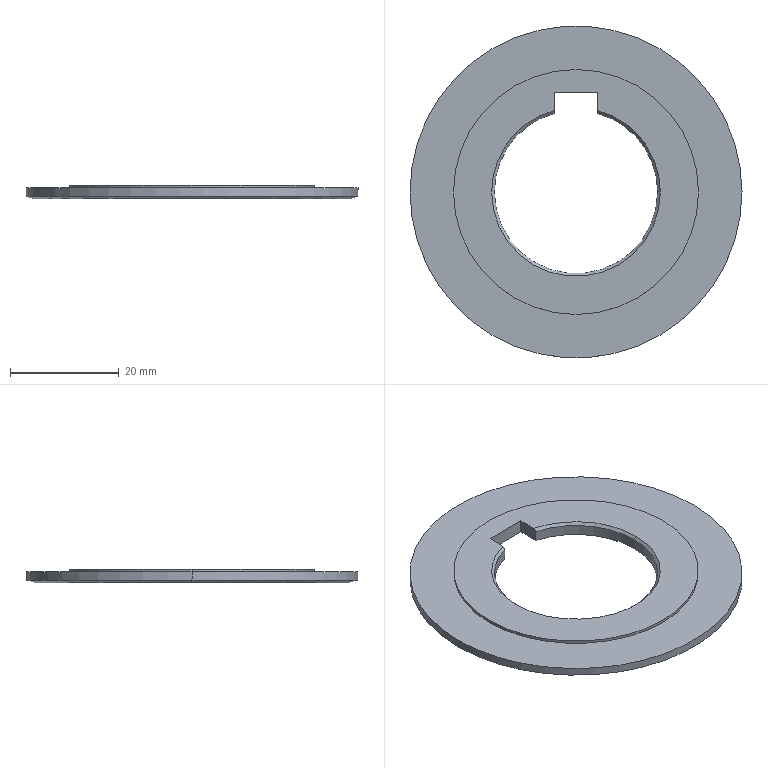Part | SolidWorks | features ICE 2, BaseBody 1 | 1 solid | 18 faces | box 61 x 61 x 2.5 mm | volume 4721 mm3 | cylinder 7 | plane 6 | cone 5 | commonest cylinder face diameters 30 x3 45 x2 61 x2
STEP:
#1=CARTESIAN_POINT('',(15.,0.,-0.5));
#2=VERTEX_POINT('',#1);
#3=CARTESIAN_POINT('',(-15.,0.,-0.5));
#4=VERTEX_POINT('',#3);
#5=CARTESIAN_POINT('',(0.,0.,-0.5));
#6=DIRECTION('',(0.,0.,-1.));
#7=DIRECTION('',(-1.,0.,0.));
#8=AXIS2_PLACEMENT_3D('',#5,#6,#7);
#9=CIRCLE('',#8,15.);
#10=EDGE_CURVE('',#2,#4,#9,.T.);
#11=ORIENTED_EDGE('',*,*,#10,.T.);
#12=CARTESIAN_POINT('',(-15.5,0.,0.));
#13=VERTEX_POINT('',#12);
#14=CARTESIAN_POINT('',(-15.5,0.,0.));
#15=DIRECTION('',(-0.7071,0.,0.7071));
#16=VECTOR('',#15,1000.);
#17=LINE('',#14,#16);
#18=EDGE_CURVE('',#4,#13,#17,.T.);
#19=ORIENTED_EDGE('',*,*,#18,.T.);
#20=CARTESIAN_POINT('',(15.5,0.,0.));
#21=VERTEX_POINT('',#20);
#22=CARTESIAN_POINT('',(0.,0.,0.));
#23=DIRECTION('',(0.,0.,-1.));
#24=DIRECTION('',(1.,0.,0.));
#25=AXIS2_PLACEMENT_3D('',#22,#23,#24);
#26=CIRCLE('',#25,15.5);
#27=EDGE_CURVE('',#21,#13,#26,.T.);
#28=ORIENTED_EDGE('',*,*,#27,.F.);
#29=CARTESIAN_POINT('',(15.5,0.,0.));
#30=DIRECTION('',(0.7071,0.,0.7071));
#31=VECTOR('',#30,1000.);
#32=LINE('',#29,#31);
#33=EDGE_CURVE('',#2,#21,#32,.T.);
#34=ORIENTED_EDGE('',*,*,#33,.F.);
#35=EDGE_LOOP('',(#11,#19,#28,#34));
#36=FACE_OUTER_BOUND('',#35,.T.);
#37=CARTESIAN_POINT('',(0.,0.,0.));
#38=DIRECTION('',(0.,0.,1.));
#39=DIRECTION('',(1.,0.,0.));
#40=AXIS2_PLACEMENT_3D('',#37,#38,#39);
#41=CONICAL_SURFACE('',#40,15.5,0.7854);
#42=ADVANCED_FACE('',(#36),#41,.F.);
#43=CARTESIAN_POINT('',(4.,14.457,-0.5));
#44=VERTEX_POINT('',#43);
#45=CARTESIAN_POINT('',(0.,0.,-0.5));
#46=DIRECTION('',(0.,0.,-1.));
#47=DIRECTION('',(-1.,0.,0.));
#48=AXIS2_PLACEMENT_3D('',#45,#46,#47);
#49=CIRCLE('',#48,15.);
#50=EDGE_CURVE('',#44,#2,#49,.T.);
#51=ORIENTED_EDGE('',*,*,#50,.T.);
#52=ORIENTED_EDGE('',*,*,#33,.T.);
#53=CARTESIAN_POINT('',(4.,14.975,0.));
#54=VERTEX_POINT('',#53);
#55=CARTESIAN_POINT('',(0.,0.,0.));
#56=DIRECTION('',(0.,0.,-1.));
#57=DIRECTION('',(1.,0.,0.));
#58=AXIS2_PLACEMENT_3D('',#55,#56,#57);
#59=CIRCLE('',#58,15.5);
#60=EDGE_CURVE('',#54,#21,#59,.T.);
#61=ORIENTED_EDGE('',*,*,#60,.F.);
#62=CARTESIAN_POINT('',(4.,14.975,0.));
#63=CARTESIAN_POINT('',(4.,14.802,-0.1668));
#64=CARTESIAN_POINT('',(4.,14.63,-0.3334));
#65=CARTESIAN_POINT('',(4.,14.457,-0.5));
#66=B_SPLINE_CURVE_WITH_KNOTS('',3,(#62,#63,#64,#65),.UNSPECIFIED.,.F.,.F.,(4,4),(0.001663,0.002383),.UNSPECIFIED.);
#67=EDGE_CURVE('',#54,#44,#66,.T.);
#68=ORIENTED_EDGE('',*,*,#67,.T.);
#69=EDGE_LOOP('',(#51,#52,#61,#68));
#70=FACE_OUTER_BOUND('',#69,.T.);
#71=CARTESIAN_POINT('',(0.,0.,0.));
#72=DIRECTION('',(0.,0.,1.));
#73=DIRECTION('',(1.,0.,0.));
#74=AXIS2_PLACEMENT_3D('',#71,#72,#73);
#75=CONICAL_SURFACE('',#74,15.5,0.7854);
#76=ADVANCED_FACE('',(#70),#75,.F.);
#77=CARTESIAN_POINT('',(-22.5,0.,0.));
#78=VERTEX_POINT('',#77);
#79=CARTESIAN_POINT('',(22.5,0.,0.));
#80=VERTEX_POINT('',#79);
#81=CARTESIAN_POINT('',(0.,0.,0.));
#82=DIRECTION('',(0.,0.,-1.));
#83=DIRECTION('',(-1.,0.,0.));
#84=AXIS2_PLACEMENT_3D('',#81,#82,#83);
#85=CIRCLE('',#84,22.5);
#86=EDGE_CURVE('',#78,#80,#85,.T.);
#87=ORIENTED_EDGE('',*,*,#86,.T.);
#88=CARTESIAN_POINT('',(22.5,0.,-0.5));
#89=VERTEX_POINT('',#88);
#90=CARTESIAN_POINT('',(22.5,0.,-49.));
#91=DIRECTION('',(0.,0.,-1.));
#92=VECTOR('',#91,1000.);
#93=LINE('',#90,#92);
#94=EDGE_CURVE('',#80,#89,#93,.T.);
#95=ORIENTED_EDGE('',*,*,#94,.T.);
#96=CARTESIAN_POINT('',(-22.5,0.,-0.5));
#97=VERTEX_POINT('',#96);
#98=CARTESIAN_POINT('',(0.,0.,-0.5));
#99=DIRECTION('',(0.,0.,1.));
#100=DIRECTION('',(-1.,0.,0.));
#101=AXIS2_PLACEMENT_3D('',#98,#99,#100);
#102=CIRCLE('',#101,22.5);
#103=EDGE_CURVE('',#89,#97,#102,.T.);
#104=ORIENTED_EDGE('',*,*,#103,.T.);
#105=CARTESIAN_POINT('',(-22.5,0.,-49.));
#106=DIRECTION('',(0.,0.,-1.));
#107=VECTOR('',#106,1000.);
#108=LINE('',#105,#107);
#109=EDGE_CURVE('',#78,#97,#108,.T.);
#110=ORIENTED_EDGE('',*,*,#109,.F.);
#111=EDGE_LOOP('',(#87,#95,#104,#110));
#112=FACE_OUTER_BOUND('',#111,.T.);
#113=CARTESIAN_POINT('',(0.,0.,-49.));
#114=DIRECTION('',(0.,0.,-1.));
#115=DIRECTION('',(-1.,0.,0.));
#116=AXIS2_PLACEMENT_3D('',#113,#114,#115);
#117=CYLINDRICAL_SURFACE('',#116,22.5);
#118=ADVANCED_FACE('',(#112),#117,.T.);
#119=CARTESIAN_POINT('',(30.5,0.,-0.5));
#120=VERTEX_POINT('',#119);
#121=CARTESIAN_POINT('',(-30.5,0.,-0.5));
#122=VERTEX_POINT('',#121);
#123=CARTESIAN_POINT('',(0.,0.,-0.5));
#124=DIRECTION('',(0.,0.,1.));
#125=DIRECTION('',(-1.,0.,0.));
#126=AXIS2_PLACEMENT_3D('',#123,#124,#125);
#127=CIRCLE('',#126,30.5);
#128=EDGE_CURVE('',#120,#122,#127,.T.);
#129=ORIENTED_EDGE('',*,*,#128,.F.);
#130=CARTESIAN_POINT('',(30.5,0.,-2.));
#131=VERTEX_POINT('',#130);
#132=CARTESIAN_POINT('',(30.5,0.,-500.));
#133=DIRECTION('',(0.,0.,-1.));
#134=VECTOR('',#133,1000.);
#135=LINE('',#132,#134);
#136=EDGE_CURVE('',#120,#131,#135,.T.);
#137=ORIENTED_EDGE('',*,*,#136,.T.);
#138=CARTESIAN_POINT('',(-30.5,0.,-2.));
#139=VERTEX_POINT('',#138);
#140=CARTESIAN_POINT('',(0.,0.,-2.));
#141=DIRECTION('',(0.,0.,1.));
#142=DIRECTION('',(-1.,0.,0.));
#143=AXIS2_PLACEMENT_3D('',#140,#141,#142);
#144=CIRCLE('',#143,30.5);
#145=EDGE_CURVE('',#131,#139,#144,.T.);
#146=ORIENTED_EDGE('',*,*,#145,.T.);
#147=CARTESIAN_POINT('',(-30.5,0.,-500.));
#148=DIRECTION('',(0.,0.,-1.));
#149=VECTOR('',#148,1000.);
#150=LINE('',#147,#149);
#151=EDGE_CURVE('',#122,#139,#150,.T.);
#152=ORIENTED_EDGE('',*,*,#151,.F.);
#153=EDGE_LOOP('',(#129,#137,#146,#152));
#154=FACE_OUTER_BOUND('',#153,.T.);
#155=CARTESIAN_POINT('',(0.,0.,-500.));
#156=DIRECTION('',(0.,0.,-1.));
#157=DIRECTION('',(-1.,0.,0.));
#158=AXIS2_PLACEMENT_3D('',#155,#156,#157);
#159=CYLINDRICAL_SURFACE('',#158,30.5);
#160=ADVANCED_FACE('',(#154),#159,.T.);
#161=CARTESIAN_POINT('',(29.,0.,-2.5));
#162=VERTEX_POINT('',#161);
#163=CARTESIAN_POINT('',(-29.,0.,-2.5));
#164=VERTEX_POINT('',#163);
#165=CARTESIAN_POINT('',(0.,0.,-2.5));
#166=DIRECTION('',(0.,0.,1.));
#167=DIRECTION('',(1.,0.,0.));
#168=AXIS2_PLACEMENT_3D('',#165,#166,#167);
#169=CIRCLE('',#168,29.);
#170=EDGE_CURVE('',#162,#164,#169,.T.);
#171=ORIENTED_EDGE('',*,*,#170,.T.);
#172=CARTESIAN_POINT('',(-30.5,0.,-2.));
#173=DIRECTION('',(-0.9487,0.,0.3162));
#174=VECTOR('',#173,1000.);
#175=LINE('',#172,#174);
#176=EDGE_CURVE('',#164,#139,#175,.T.);
#177=ORIENTED_EDGE('',*,*,#176,.T.);
#178=ORIENTED_EDGE('',*,*,#145,.F.);
#179=CARTESIAN_POINT('',(30.5,0.,-2.));
#180=DIRECTION('',(0.9487,0.,0.3162));
#181=VECTOR('',#180,1000.);
#182=LINE('',#179,#181);
#183=EDGE_CURVE('',#162,#131,#182,.T.);
#184=ORIENTED_EDGE('',*,*,#183,.F.);
#185=EDGE_LOOP('',(#171,#177,#178,#184));
#186=FACE_OUTER_BOUND('',#185,.T.);
#187=CARTESIAN_POINT('',(0.,0.,-2.));
#188=DIRECTION('',(0.,0.,1.));
#189=DIRECTION('',(1.,0.,0.));
#190=AXIS2_PLACEMENT_3D('',#187,#188,#189);
#191=CONICAL_SURFACE('',#190,30.5,1.249);
#192=ADVANCED_FACE('',(#186),#191,.T.);
#193=ORIENTED_EDGE('',*,*,#10,.F.);
#194=CARTESIAN_POINT('',(15.,0.,-2.5));
#195=VERTEX_POINT('',#194);
#196=CARTESIAN_POINT('',(15.,0.,-49.));
#197=DIRECTION('',(0.,0.,-1.));
#198=VECTOR('',#197,1000.);
#199=LINE('',#196,#198);
#200=EDGE_CURVE('',#2,#195,#199,.T.);
#201=ORIENTED_EDGE('',*,*,#200,.T.);
#202=CARTESIAN_POINT('',(-15.,0.,-2.5));
#203=VERTEX_POINT('',#202);
#204=CARTESIAN_POINT('',(0.,0.,-2.5));
#205=DIRECTION('',(0.,0.,1.));
#206=DIRECTION('',(-1.,0.,0.));
#207=AXIS2_PLACEMENT_3D('',#204,#205,#206);
#208=CIRCLE('',#207,15.);
#209=EDGE_CURVE('',#203,#195,#208,.T.);
#210=ORIENTED_EDGE('',*,*,#209,.F.);
#211=CARTESIAN_POINT('',(-15.,0.,-49.));
#212=DIRECTION('',(0.,0.,-1.));
#213=VECTOR('',#212,1000.);
#214=LINE('',#211,#213);
#215=EDGE_CURVE('',#4,#203,#214,.T.);
#216=ORIENTED_EDGE('',*,*,#215,.F.);
#217=EDGE_LOOP('',(#193,#201,#210,#216));
#218=FACE_OUTER_BOUND('',#217,.T.);
#219=CARTESIAN_POINT('',(0.,0.,-49.));
#220=DIRECTION('',(0.,0.,-1.));
#221=DIRECTION('',(-1.,0.,0.));
#222=AXIS2_PLACEMENT_3D('',#219,#220,#221);
#223=CYLINDRICAL_SURFACE('',#222,15.);
#224=ADVANCED_FACE('',(#218),#223,.F.);
#225=CARTESIAN_POINT('',(-4.,14.457,-0.5));
#226=VERTEX_POINT('',#225);
#227=CARTESIAN_POINT('',(0.,0.,-0.5));
#228=DIRECTION('',(0.,0.,-1.));
#229=DIRECTION('',(-1.,0.,0.));
#230=AXIS2_PLACEMENT_3D('',#227,#228,#229);
#231=CIRCLE('',#230,15.);
#232=EDGE_CURVE('',#4,#226,#231,.T.);
#233=ORIENTED_EDGE('',*,*,#232,.F.);
#234=ORIENTED_EDGE('',*,*,#215,.T.);
#235=CARTESIAN_POINT('',(-4.,14.457,-2.5));
#236=VERTEX_POINT('',#235);
#237=CARTESIAN_POINT('',(0.,0.,-2.5));
#238=DIRECTION('',(0.,0.,1.));
#239=DIRECTION('',(-1.,0.,0.));
#240=AXIS2_PLACEMENT_3D('',#237,#238,#239);
#241=CIRCLE('',#240,15.);
#242=EDGE_CURVE('',#236,#203,#241,.T.);
#243=ORIENTED_EDGE('',*,*,#242,.F.);
#244=CARTESIAN_POINT('',(-4.,14.457,-11.393));
#245=DIRECTION('',(0.,0.,1.));
#246=VECTOR('',#245,1000.);
#247=LINE('',#244,#246);
#248=EDGE_CURVE('',#236,#226,#247,.T.);
#249=ORIENTED_EDGE('',*,*,#248,.T.);
#250=EDGE_LOOP('',(#233,#234,#243,#249));
#251=FACE_OUTER_BOUND('',#250,.T.);
#252=CARTESIAN_POINT('',(0.,0.,-49.));
#253=DIRECTION('',(0.,0.,-1.));
#254=DIRECTION('',(-1.,0.,0.));
#255=AXIS2_PLACEMENT_3D('',#252,#253,#254);
#256=CYLINDRICAL_SURFACE('',#255,15.);
#257=ADVANCED_FACE('',(#251),#256,.F.);
#258=ORIENTED_EDGE('',*,*,#200,.F.);
#259=ORIENTED_EDGE('',*,*,#50,.F.);
#260=CARTESIAN_POINT('',(4.,14.457,-2.5));
#261=VERTEX_POINT('',#260);
#262=CARTESIAN_POINT('',(4.,14.457,-11.393));
#263=DIRECTION('',(0.,0.,1.));
#264=VECTOR('',#263,1000.);
#265=LINE('',#262,#264);
#266=EDGE_CURVE('',#261,#44,#265,.T.);
#267=ORIENTED_EDGE('',*,*,#266,.F.);
#268=CARTESIAN_POINT('',(0.,0.,-2.5));
#269=DIRECTION('',(0.,0.,1.));
#270=DIRECTION('',(-1.,0.,0.));
#271=AXIS2_PLACEMENT_3D('',#268,#269,#270);
#272=CIRCLE('',#271,15.);
#273=EDGE_CURVE('',#195,#261,#272,.T.);
#274=ORIENTED_EDGE('',*,*,#273,.F.);
#275=EDGE_LOOP('',(#258,#259,#267,#274));
#276=FACE_OUTER_BOUND('',#275,.T.);
#277=CARTESIAN_POINT('',(0.,0.,-49.));
#278=DIRECTION('',(0.,0.,-1.));
#279=DIRECTION('',(-1.,0.,0.));
#280=AXIS2_PLACEMENT_3D('',#277,#278,#279);
#281=CYLINDRICAL_SURFACE('',#280,15.);
#282=ADVANCED_FACE('',(#276),#281,.F.);
#283=ORIENTED_EDGE('',*,*,#18,.F.);
#284=ORIENTED_EDGE('',*,*,#232,.T.);
#285=CARTESIAN_POINT('',(-4.,14.975,0.));
#286=VERTEX_POINT('',#285);
#287=CARTESIAN_POINT('',(-4.,14.457,-0.5));
#288=CARTESIAN_POINT('',(-4.,14.63,-0.3334));
#289=CARTESIAN_POINT('',(-4.,14.802,-0.1668));
#290=CARTESIAN_POINT('',(-4.,14.975,0.));
#291=B_SPLINE_CURVE_WITH_KNOTS('',3,(#287,#288,#289,#290),.UNSPECIFIED.,.F.,.F.,(4,4),(0.001605,0.002325),.UNSPECIFIED.);
#292=EDGE_CURVE('',#226,#286,#291,.T.);
#293=ORIENTED_EDGE('',*,*,#292,.T.);
#294=CARTESIAN_POINT('',(0.,0.,0.));
#295=DIRECTION('',(0.,0.,-1.));
#296=DIRECTION('',(1.,0.,0.));
#297=AXIS2_PLACEMENT_3D('',#294,#295,#296);
#298=CIRCLE('',#297,15.5);
#299=EDGE_CURVE('',#13,#286,#298,.T.);
#300=ORIENTED_EDGE('',*,*,#299,.F.);
#301=EDGE_LOOP('',(#283,#284,#293,#300));
#302=FACE_OUTER_BOUND('',#301,.T.);
#303=CARTESIAN_POINT('',(0.,0.,0.));
#304=DIRECTION('',(0.,0.,1.));
#305=DIRECTION('',(1.,0.,0.));
#306=AXIS2_PLACEMENT_3D('',#303,#304,#305);
#307=CONICAL_SURFACE('',#306,15.5,0.7854);
#308=ADVANCED_FACE('',(#302),#307,.F.);
#309=CARTESIAN_POINT('',(4.,18.34,0.));
#310=VERTEX_POINT('',#309);
#311=CARTESIAN_POINT('',(-4.,18.34,0.));
#312=VERTEX_POINT('',#311);
#313=CARTESIAN_POINT('',(-4.,18.34,0.));
#314=DIRECTION('',(-1.,0.,0.));
#315=VECTOR('',#314,1000.);
#316=LINE('',#313,#315);
#317=EDGE_CURVE('',#310,#312,#316,.T.);
#318=ORIENTED_EDGE('',*,*,#317,.F.);
#319=CARTESIAN_POINT('',(4.,18.34,0.));
#320=DIRECTION('',(0.,1.,0.));
#321=VECTOR('',#320,1000.);
#322=LINE('',#319,#321);
#323=EDGE_CURVE('',#54,#310,#322,.T.);
#324=ORIENTED_EDGE('',*,*,#323,.F.);
#325=ORIENTED_EDGE('',*,*,#60,.T.);
#326=ORIENTED_EDGE('',*,*,#27,.T.);
#327=ORIENTED_EDGE('',*,*,#299,.T.);
#328=CARTESIAN_POINT('',(-4.,18.34,0.));
#329=DIRECTION('',(0.,-1.,0.));
#330=VECTOR('',#329,1000.);
#331=LINE('',#328,#330);
#332=EDGE_CURVE('',#312,#286,#331,.T.);
#333=ORIENTED_EDGE('',*,*,#332,.F.);
#334=EDGE_LOOP('',(#318,#324,#325,#326,#327,#333));
#335=FACE_BOUND('',#334,.T.);
#336=ORIENTED_EDGE('',*,*,#86,.F.);
#337=CARTESIAN_POINT('',(0.,0.,0.));
#338=DIRECTION('',(0.,0.,-1.));
#339=DIRECTION('',(-1.,0.,0.));
#340=AXIS2_PLACEMENT_3D('',#337,#338,#339);
#341=CIRCLE('',#340,22.5);
#342=EDGE_CURVE('',#80,#78,#341,.T.);
#343=ORIENTED_EDGE('',*,*,#342,.F.);
#344=EDGE_LOOP('',(#336,#343));
#345=FACE_OUTER_BOUND('',#344,.T.);
#346=CARTESIAN_POINT('',(0.,0.,0.));
#347=DIRECTION('',(0.,0.,-1.));
#348=DIRECTION('',(-1.,0.,0.));
#349=AXIS2_PLACEMENT_3D('',#346,#347,#348);
#350=PLANE('',#349);
#351=ADVANCED_FACE('',(#335,#345),#350,.F.);
#352=ORIENTED_EDGE('',*,*,#94,.F.);
#353=ORIENTED_EDGE('',*,*,#342,.T.);
#354=ORIENTED_EDGE('',*,*,#109,.T.);
#355=CARTESIAN_POINT('',(0.,0.,-0.5));
#356=DIRECTION('',(0.,0.,1.));
#357=DIRECTION('',(-1.,0.,0.));
#358=AXIS2_PLACEMENT_3D('',#355,#356,#357);
#359=CIRCLE('',#358,22.5);
#360=EDGE_CURVE('',#97,#89,#359,.T.);
#361=ORIENTED_EDGE('',*,*,#360,.T.);
#362=EDGE_LOOP('',(#352,#353,#354,#361));
#363=FACE_OUTER_BOUND('',#362,.T.);
#364=CARTESIAN_POINT('',(0.,0.,-49.));
#365=DIRECTION('',(0.,0.,-1.));
#366=DIRECTION('',(-1.,0.,0.));
#367=AXIS2_PLACEMENT_3D('',#364,#365,#366);
#368=CYLINDRICAL_SURFACE('',#367,22.5);
#369=ADVANCED_FACE('',(#363),#368,.T.);
#370=CARTESIAN_POINT('',(0.,0.,-0.5));
#371=DIRECTION('',(0.,0.,1.));
#372=DIRECTION('',(-1.,0.,0.));
#373=AXIS2_PLACEMENT_3D('',#370,#371,#372);
#374=CIRCLE('',#373,30.5);
#375=EDGE_CURVE('',#122,#120,#374,.T.);
#376=ORIENTED_EDGE('',*,*,#375,.T.);
#377=ORIENTED_EDGE('',*,*,#128,.T.);
#378=EDGE_LOOP('',(#376,#377));
#379=FACE_OUTER_BOUND('',#378,.T.);
#380=ORIENTED_EDGE('',*,*,#360,.F.);
#381=ORIENTED_EDGE('',*,*,#103,.F.);
#382=EDGE_LOOP('',(#380,#381));
#383=FACE_BOUND('',#382,.T.);
#384=CARTESIAN_POINT('',(0.,30.5,-0.5));
#385=DIRECTION('',(0.,0.,1.));
#386=DIRECTION('',(1.,0.,0.));
#387=AXIS2_PLACEMENT_3D('',#384,#385,#386);
#388=PLANE('',#387);
#389=ADVANCED_FACE('',(#379,#383),#388,.T.);
#390=ORIENTED_EDGE('',*,*,#136,.F.);
#391=ORIENTED_EDGE('',*,*,#375,.F.);
#392=ORIENTED_EDGE('',*,*,#151,.T.);
#393=CARTESIAN_POINT('',(0.,0.,-2.));
#394=DIRECTION('',(0.,0.,1.));
#395=DIRECTION('',(-1.,0.,0.));
#396=AXIS2_PLACEMENT_3D('',#393,#394,#395);
#397=CIRCLE('',#396,30.5);
#398=EDGE_CURVE('',#139,#131,#397,.T.);
#399=ORIENTED_EDGE('',*,*,#398,.T.);
#400=EDGE_LOOP('',(#390,#391,#392,#399));
#401=FACE_OUTER_BOUND('',#400,.T.);
#402=CARTESIAN_POINT('',(0.,0.,-500.));
#403=DIRECTION('',(0.,0.,-1.));
#404=DIRECTION('',(-1.,0.,0.));
#405=AXIS2_PLACEMENT_3D('',#402,#403,#404);
#406=CYLINDRICAL_SURFACE('',#405,30.5);
#407=ADVANCED_FACE('',(#401),#406,.T.);
#408=ORIENTED_EDGE('',*,*,#176,.F.);
#409=CARTESIAN_POINT('',(0.,0.,-2.5));
#410=DIRECTION('',(0.,0.,1.));
#411=DIRECTION('',(1.,0.,0.));
#412=AXIS2_PLACEMENT_3D('',#409,#410,#411);
#413=CIRCLE('',#412,29.);
#414=EDGE_CURVE('',#164,#162,#413,.T.);
#415=ORIENTED_EDGE('',*,*,#414,.T.);
#416=ORIENTED_EDGE('',*,*,#183,.T.);
#417=ORIENTED_EDGE('',*,*,#398,.F.);
#418=EDGE_LOOP('',(#408,#415,#416,#417));
#419=FACE_OUTER_BOUND('',#418,.T.);
#420=CARTESIAN_POINT('',(0.,0.,-2.));
#421=DIRECTION('',(0.,0.,1.));
#422=DIRECTION('',(1.,0.,0.));
#423=AXIS2_PLACEMENT_3D('',#420,#421,#422);
#424=CONICAL_SURFACE('',#423,30.5,1.249);
#425=ADVANCED_FACE('',(#419),#424,.T.);
#426=CARTESIAN_POINT('',(4.,18.34,-2.5));
#427=VERTEX_POINT('',#426);
#428=CARTESIAN_POINT('',(4.,18.34,-2.5));
#429=DIRECTION('',(0.,1.,0.));
#430=VECTOR('',#429,1000.);
#431=LINE('',#428,#430);
#432=EDGE_CURVE('',#261,#427,#431,.T.);
#433=ORIENTED_EDGE('',*,*,#432,.T.);
#434=CARTESIAN_POINT('',(-4.,18.34,-2.5));
#435=VERTEX_POINT('',#434);
#436=CARTESIAN_POINT('',(-4.,18.34,-2.5));
#437=DIRECTION('',(-1.,0.,0.));
#438=VECTOR('',#437,1000.);
#439=LINE('',#436,#438);
#440=EDGE_CURVE('',#427,#435,#439,.T.);
#441=ORIENTED_EDGE('',*,*,#440,.T.);
#442=CARTESIAN_POINT('',(-4.,18.34,-2.5));
#443=DIRECTION('',(0.,-1.,0.));
#444=VECTOR('',#443,1000.);
#445=LINE('',#442,#444);
#446=EDGE_CURVE('',#435,#236,#445,.T.);
#447=ORIENTED_EDGE('',*,*,#446,.T.);
#448=ORIENTED_EDGE('',*,*,#242,.T.);
#449=ORIENTED_EDGE('',*,*,#209,.T.);
#450=ORIENTED_EDGE('',*,*,#273,.T.);
#451=EDGE_LOOP('',(#433,#441,#447,#448,#449,#450));
#452=FACE_BOUND('',#451,.T.);
#453=ORIENTED_EDGE('',*,*,#170,.F.);
#454=ORIENTED_EDGE('',*,*,#414,.F.);
#455=EDGE_LOOP('',(#453,#454));
#456=FACE_OUTER_BOUND('',#455,.T.);
#457=CARTESIAN_POINT('',(0.,22.5,-2.5));
#458=DIRECTION('',(0.,0.,-1.));
#459=DIRECTION('',(-1.,0.,0.));
#460=AXIS2_PLACEMENT_3D('',#457,#458,#459);
#461=PLANE('',#460);
#462=ADVANCED_FACE('',(#452,#456),#461,.T.);
#463=ORIENTED_EDGE('',*,*,#323,.T.);
#464=CARTESIAN_POINT('',(4.,18.34,-11.393));
#465=DIRECTION('',(0.,0.,1.));
#466=VECTOR('',#465,1000.);
#467=LINE('',#464,#466);
#468=EDGE_CURVE('',#427,#310,#467,.T.);
#469=ORIENTED_EDGE('',*,*,#468,.F.);
#470=ORIENTED_EDGE('',*,*,#432,.F.);
#471=ORIENTED_EDGE('',*,*,#266,.T.);
#472=ORIENTED_EDGE('',*,*,#67,.F.);
#473=EDGE_LOOP('',(#463,#469,#470,#471,#472));
#474=FACE_OUTER_BOUND('',#473,.T.);
#475=CARTESIAN_POINT('',(4.,18.34,-11.393));
#476=DIRECTION('',(1.,0.,0.));
#477=DIRECTION('',(0.,0.,-1.));
#478=AXIS2_PLACEMENT_3D('',#475,#476,#477);
#479=PLANE('',#478);
#480=ADVANCED_FACE('',(#474),#479,.F.);
#481=ORIENTED_EDGE('',*,*,#248,.F.);
#482=ORIENTED_EDGE('',*,*,#446,.F.);
#483=CARTESIAN_POINT('',(-4.,18.34,-11.393));
#484=DIRECTION('',(0.,0.,1.));
#485=VECTOR('',#484,1000.);
#486=LINE('',#483,#485);
#487=EDGE_CURVE('',#435,#312,#486,.T.);
#488=ORIENTED_EDGE('',*,*,#487,.T.);
#489=ORIENTED_EDGE('',*,*,#332,.T.);
#490=ORIENTED_EDGE('',*,*,#292,.F.);
#491=EDGE_LOOP('',(#481,#482,#488,#489,#490));
#492=FACE_OUTER_BOUND('',#491,.T.);
#493=CARTESIAN_POINT('',(-4.,18.34,-11.393));
#494=DIRECTION('',(-1.,0.,0.));
#495=DIRECTION('',(0.,0.,1.));
#496=AXIS2_PLACEMENT_3D('',#493,#494,#495);
#497=PLANE('',#496);
#498=ADVANCED_FACE('',(#492),#497,.F.);
#499=ORIENTED_EDGE('',*,*,#468,.T.);
#500=ORIENTED_EDGE('',*,*,#317,.T.);
#501=ORIENTED_EDGE('',*,*,#487,.F.);
#502=ORIENTED_EDGE('',*,*,#440,.F.);
#503=EDGE_LOOP('',(#499,#500,#501,#502));
#504=FACE_OUTER_BOUND('',#503,.T.);
#505=CARTESIAN_POINT('',(-4.,18.34,-11.393));
#506=DIRECTION('',(0.,1.,0.));
#507=DIRECTION('',(0.,0.,1.));
#508=AXIS2_PLACEMENT_3D('',#505,#506,#507);
#509=PLANE('',#508);
#510=ADVANCED_FACE('',(#504),#509,.F.);
#511=CLOSED_SHELL('',(#42,#76,#118,#160,#192,#224,#257,#282,#308,#351,#369,#389,#407,#425,#462,#480,#498,#510));
#512=MANIFOLD_SOLID_BREP('',#511);
#513=CARTESIAN_POINT('',(0.,0.,0.));
#514=DIRECTION('',(0.,0.,1.));
#515=DIRECTION('',(1.,0.,0.));
#516=AXIS2_PLACEMENT_3D('',#513,#514,#515);
#517=(LENGTH_UNIT()NAMED_UNIT(*)SI_UNIT(.MILLI.,.METRE.));
#518=UNCERTAINTY_MEASURE_WITH_UNIT(LENGTH_MEASURE(0.00001),#517,'','');
#519=(NAMED_UNIT(*)PLANE_ANGLE_UNIT()SI_UNIT($,.RADIAN.));
#520=(NAMED_UNIT(*)SI_UNIT($,.STERADIAN.)SOLID_ANGLE_UNIT());
#521=(GEOMETRIC_REPRESENTATION_CONTEXT(3)GLOBAL_UNCERTAINTY_ASSIGNED_CONTEXT((#518))GLOBAL_UNIT_ASSIGNED_CONTEXT((#517,#519,#520))REPRESENTATION_CONTEXT('',''));
#522=ADVANCED_BREP_SHAPE_REPRESENTATION('',(#512,#516),#521);